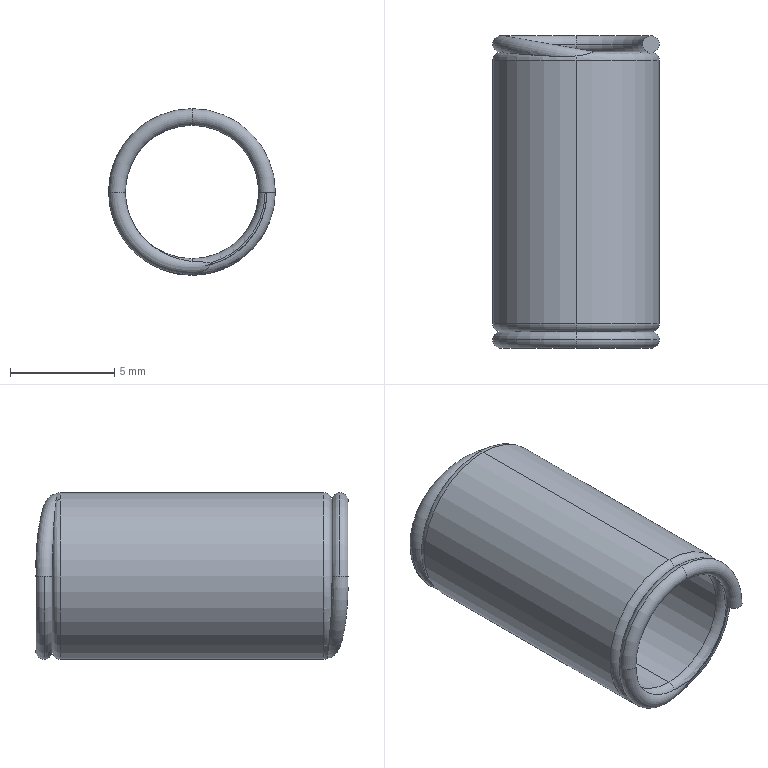Part | STEP file | 11-WT8_1511 | 1 solid | 30 faces | box 8 x 15 x 8 mm | volume 255.021 mm3 | torus 22 | cylinder 4 | plane 4 | commonest cylinder face diameters 6.4 x2 8 x2
STEP:
#1=CARTESIAN_POINT('',(0.,-7.1,4.));
#2=VERTEX_POINT('',#1);
#3=CARTESIAN_POINT('',(0.,-7.1,3.2));
#4=VERTEX_POINT('',#3);
#5=CARTESIAN_POINT('',(0.,-7.1,3.6));
#6=DIRECTION('',(1.,0.,0.));
#7=DIRECTION('',(0.,0.,-1.));
#8=AXIS2_PLACEMENT_3D('',#5,#6,#7);
#9=CIRCLE('',#8,0.4);
#10=EDGE_CURVE('',#2,#4,#9,.T.);
#11=ORIENTED_EDGE('',*,*,#10,.F.);
#12=CARTESIAN_POINT('',(-4.,-7.1,0.));
#13=VERTEX_POINT('',#12);
#14=CARTESIAN_POINT('',(0.,-7.1,0.));
#15=DIRECTION('',(0.,-1.,0.));
#16=DIRECTION('',(0.,0.,-1.));
#17=AXIS2_PLACEMENT_3D('',#14,#15,#16);
#18=CIRCLE('',#17,4.);
#19=EDGE_CURVE('',#2,#13,#18,.T.);
#20=ORIENTED_EDGE('',*,*,#19,.T.);
#21=CARTESIAN_POINT('',(-3.2,-7.1,0.));
#22=VERTEX_POINT('',#21);
#23=CARTESIAN_POINT('',(-3.6,-7.1,0.));
#24=DIRECTION('',(0.,0.,1.));
#25=DIRECTION('',(1.,0.,0.));
#26=AXIS2_PLACEMENT_3D('',#23,#24,#25);
#27=CIRCLE('',#26,0.4);
#28=EDGE_CURVE('',#13,#22,#27,.T.);
#29=ORIENTED_EDGE('',*,*,#28,.T.);
#30=CARTESIAN_POINT('',(0.,-7.1,0.));
#31=DIRECTION('',(0.,-1.,0.));
#32=DIRECTION('',(0.,0.,-1.));
#33=AXIS2_PLACEMENT_3D('',#30,#31,#32);
#34=CIRCLE('',#33,3.2);
#35=EDGE_CURVE('',#4,#22,#34,.T.);
#36=ORIENTED_EDGE('',*,*,#35,.F.);
#37=EDGE_LOOP('',(#11,#20,#29,#36));
#38=FACE_OUTER_BOUND('',#37,.T.);
#39=CARTESIAN_POINT('',(0.,-7.1,0.));
#40=DIRECTION('',(0.,-1.,0.));
#41=DIRECTION('',(0.,0.,-1.));
#42=AXIS2_PLACEMENT_3D('',#39,#40,#41);
#43=TOROIDAL_SURFACE('',#42,3.6,0.4);
#44=ADVANCED_FACE('',(#38),#43,.T.);
#45=CARTESIAN_POINT('',(0.,-6.7,3.6));
#46=VERTEX_POINT('',#45);
#47=CARTESIAN_POINT('',(0.,-7.1,3.6));
#48=DIRECTION('',(1.,0.,0.));
#49=DIRECTION('',(0.,0.,-1.));
#50=AXIS2_PLACEMENT_3D('',#47,#48,#49);
#51=CIRCLE('',#50,0.4);
#52=EDGE_CURVE('',#4,#46,#51,.T.);
#53=ORIENTED_EDGE('',*,*,#52,.F.);
#54=ORIENTED_EDGE('',*,*,#35,.T.);
#55=CARTESIAN_POINT('',(0.,-6.807,-3.328));
#56=VERTEX_POINT('',#55);
#57=CARTESIAN_POINT('',(0.,-6.807,-3.328));
#58=CARTESIAN_POINT('',(-0.4208,-6.848,-3.284));
#59=CARTESIAN_POINT('',(-0.8292,-6.886,-3.181));
#60=CARTESIAN_POINT('',(-1.409,-6.939,-2.918));
#61=CARTESIAN_POINT('',(-1.592,-6.956,-2.814));
#62=CARTESIAN_POINT('',(-1.937,-6.987,-2.576));
#63=CARTESIAN_POINT('',(-2.101,-7.002,-2.439));
#64=CARTESIAN_POINT('',(-2.398,-7.029,-2.139));
#65=CARTESIAN_POINT('',(-2.531,-7.041,-1.976));
#66=CARTESIAN_POINT('',(-2.766,-7.062,-1.627));
#67=CARTESIAN_POINT('',(-2.868,-7.071,-1.438));
#68=CARTESIAN_POINT('',(-3.031,-7.085,-1.047));
#69=CARTESIAN_POINT('',(-3.095,-7.091,-0.8424));
#70=CARTESIAN_POINT('',(-3.179,-7.098,-0.4249));
#71=CARTESIAN_POINT('',(-3.2,-7.1,-0.2096));
#72=CARTESIAN_POINT('',(-3.2,-7.1,0.));
#73=B_SPLINE_CURVE_WITH_KNOTS('',3,(#57,#58,#59,#60,#61,#62,#63,#64,#65,#66,#67,#68,#69,#70,#71,#72),.UNSPECIFIED.,.F.,.F.,(4,2,2,2,2,2,2,4),(0.001402,0.002659,0.003288,0.003917,0.004545,0.005174,0.005803,0.006431),.UNSPECIFIED.);
#74=EDGE_CURVE('',#56,#22,#73,.T.);
#75=ORIENTED_EDGE('',*,*,#74,.F.);
#76=CARTESIAN_POINT('',(0.,-6.7,-3.6));
#77=VERTEX_POINT('',#76);
#78=CARTESIAN_POINT('',(0.,-7.1,-3.6));
#79=DIRECTION('',(-1.,0.,0.));
#80=DIRECTION('',(0.,0.,1.));
#81=AXIS2_PLACEMENT_3D('',#78,#79,#80);
#82=CIRCLE('',#81,0.4);
#83=EDGE_CURVE('',#56,#77,#82,.T.);
#84=ORIENTED_EDGE('',*,*,#83,.T.);
#85=CARTESIAN_POINT('',(0.,-6.7,0.));
#86=DIRECTION('',(0.,1.,0.));
#87=DIRECTION('',(0.,0.,1.));
#88=AXIS2_PLACEMENT_3D('',#85,#86,#87);
#89=CIRCLE('',#88,3.6);
#90=EDGE_CURVE('',#77,#46,#89,.T.);
#91=ORIENTED_EDGE('',*,*,#90,.T.);
#92=EDGE_LOOP('',(#53,#54,#75,#84,#91));
#93=FACE_OUTER_BOUND('',#92,.T.);
#94=CARTESIAN_POINT('',(0.,-7.1,0.));
#95=DIRECTION('',(0.,-1.,0.));
#96=DIRECTION('',(0.,0.,-1.));
#97=AXIS2_PLACEMENT_3D('',#94,#95,#96);
#98=TOROIDAL_SURFACE('',#97,3.6,0.4);
#99=ADVANCED_FACE('',(#93),#98,.T.);
#100=CARTESIAN_POINT('',(0.,7.1,-4.));
#101=VERTEX_POINT('',#100);
#102=CARTESIAN_POINT('',(0.,7.1,-3.2));
#103=VERTEX_POINT('',#102);
#104=CARTESIAN_POINT('',(0.,7.1,-3.6));
#105=DIRECTION('',(1.,0.,0.));
#106=DIRECTION('',(0.,0.,-1.));
#107=AXIS2_PLACEMENT_3D('',#104,#105,#106);
#108=CIRCLE('',#107,0.4);
#109=EDGE_CURVE('',#101,#103,#108,.T.);
#110=ORIENTED_EDGE('',*,*,#109,.F.);
#111=CARTESIAN_POINT('',(-4.,7.1,0.));
#112=VERTEX_POINT('',#111);
#113=CARTESIAN_POINT('',(0.,7.1,0.));
#114=DIRECTION('',(0.,1.,0.));
#115=DIRECTION('',(0.,0.,1.));
#116=AXIS2_PLACEMENT_3D('',#113,#114,#115);
#117=CIRCLE('',#116,4.);
#118=EDGE_CURVE('',#101,#112,#117,.T.);
#119=ORIENTED_EDGE('',*,*,#118,.T.);
#120=CARTESIAN_POINT('',(-3.2,7.1,0.));
#121=VERTEX_POINT('',#120);
#122=CARTESIAN_POINT('',(-3.6,7.1,0.));
#123=DIRECTION('',(0.,0.,1.));
#124=DIRECTION('',(1.,0.,0.));
#125=AXIS2_PLACEMENT_3D('',#122,#123,#124);
#126=CIRCLE('',#125,0.4);
#127=EDGE_CURVE('',#121,#112,#126,.T.);
#128=ORIENTED_EDGE('',*,*,#127,.F.);
#129=CARTESIAN_POINT('',(0.,7.1,0.));
#130=DIRECTION('',(0.,1.,0.));
#131=DIRECTION('',(0.,0.,1.));
#132=AXIS2_PLACEMENT_3D('',#129,#130,#131);
#133=CIRCLE('',#132,3.2);
#134=EDGE_CURVE('',#103,#121,#133,.T.);
#135=ORIENTED_EDGE('',*,*,#134,.F.);
#136=EDGE_LOOP('',(#110,#119,#128,#135));
#137=FACE_OUTER_BOUND('',#136,.T.);
#138=CARTESIAN_POINT('',(0.,7.1,0.));
#139=DIRECTION('',(0.,1.,0.));
#140=DIRECTION('',(0.,0.,1.));
#141=AXIS2_PLACEMENT_3D('',#138,#139,#140);
#142=TOROIDAL_SURFACE('',#141,3.6,0.4);
#143=ADVANCED_FACE('',(#137),#142,.T.);
#144=CARTESIAN_POINT('',(0.,6.7,-3.6));
#145=VERTEX_POINT('',#144);
#146=CARTESIAN_POINT('',(0.,7.1,-3.6));
#147=DIRECTION('',(1.,0.,0.));
#148=DIRECTION('',(0.,0.,-1.));
#149=AXIS2_PLACEMENT_3D('',#146,#147,#148);
#150=CIRCLE('',#149,0.4);
#151=EDGE_CURVE('',#103,#145,#150,.T.);
#152=ORIENTED_EDGE('',*,*,#151,.F.);
#153=ORIENTED_EDGE('',*,*,#134,.T.);
#154=CARTESIAN_POINT('',(0.,6.807,3.328));
#155=VERTEX_POINT('',#154);
#156=CARTESIAN_POINT('',(-3.2,7.1,0.));
#157=CARTESIAN_POINT('',(-3.2,7.1,0.4264));
#158=CARTESIAN_POINT('',(-3.113,7.092,0.8528));
#159=CARTESIAN_POINT('',(-2.867,7.071,1.439));
#160=CARTESIAN_POINT('',(-2.765,7.062,1.628));
#161=CARTESIAN_POINT('',(-2.53,7.041,1.977));
#162=CARTESIAN_POINT('',(-2.397,7.029,2.139));
#163=CARTESIAN_POINT('',(-2.1,7.002,2.439));
#164=CARTESIAN_POINT('',(-1.936,6.987,2.576));
#165=CARTESIAN_POINT('',(-1.591,6.956,2.815));
#166=CARTESIAN_POINT('',(-1.408,6.939,2.918));
#167=CARTESIAN_POINT('',(-0.829,6.886,3.181));
#168=CARTESIAN_POINT('',(-0.4207,6.848,3.284));
#169=CARTESIAN_POINT('',(0.,6.807,3.328));
#170=B_SPLINE_CURVE_WITH_KNOTS('',3,(#156,#157,#158,#159,#160,#161,#162,#163,#164,#165,#166,#167,#168,#169),.UNSPECIFIED.,.F.,.F.,(4,2,2,2,2,2,4),(-0.00008421,0.001195,0.001834,0.002474,0.003113,0.003753,0.005032),.UNSPECIFIED.);
#171=EDGE_CURVE('',#121,#155,#170,.T.);
#172=ORIENTED_EDGE('',*,*,#171,.T.);
#173=CARTESIAN_POINT('',(0.,6.7,3.6));
#174=VERTEX_POINT('',#173);
#175=CARTESIAN_POINT('',(0.,7.1,3.6));
#176=DIRECTION('',(-1.,0.,0.));
#177=DIRECTION('',(0.,0.,1.));
#178=AXIS2_PLACEMENT_3D('',#175,#176,#177);
#179=CIRCLE('',#178,0.4);
#180=EDGE_CURVE('',#155,#174,#179,.T.);
#181=ORIENTED_EDGE('',*,*,#180,.T.);
#182=CARTESIAN_POINT('',(0.,6.7,0.));
#183=DIRECTION('',(0.,1.,0.));
#184=DIRECTION('',(0.,0.,1.));
#185=AXIS2_PLACEMENT_3D('',#182,#183,#184);
#186=CIRCLE('',#185,3.6);
#187=EDGE_CURVE('',#145,#174,#186,.T.);
#188=ORIENTED_EDGE('',*,*,#187,.F.);
#189=EDGE_LOOP('',(#152,#153,#172,#181,#188));
#190=FACE_OUTER_BOUND('',#189,.T.);
#191=CARTESIAN_POINT('',(0.,7.1,0.));
#192=DIRECTION('',(0.,1.,0.));
#193=DIRECTION('',(0.,0.,1.));
#194=AXIS2_PLACEMENT_3D('',#191,#192,#193);
#195=TOROIDAL_SURFACE('',#194,3.6,0.4);
#196=ADVANCED_FACE('',(#190),#195,.T.);
#197=CARTESIAN_POINT('',(3.2,7.1,0.));
#198=VERTEX_POINT('',#197);
#199=CARTESIAN_POINT('',(4.,7.1,0.));
#200=VERTEX_POINT('',#199);
#201=CARTESIAN_POINT('',(3.6,7.1,0.));
#202=DIRECTION('',(0.,0.,-1.));
#203=DIRECTION('',(-1.,0.,0.));
#204=AXIS2_PLACEMENT_3D('',#201,#202,#203);
#205=CIRCLE('',#204,0.4);
#206=EDGE_CURVE('',#198,#200,#205,.T.);
#207=ORIENTED_EDGE('',*,*,#206,.T.);
#208=CARTESIAN_POINT('',(0.,7.1,0.));
#209=DIRECTION('',(0.,1.,0.));
#210=DIRECTION('',(0.,0.,1.));
#211=AXIS2_PLACEMENT_3D('',#208,#209,#210);
#212=CIRCLE('',#211,4.);
#213=EDGE_CURVE('',#200,#101,#212,.T.);
#214=ORIENTED_EDGE('',*,*,#213,.T.);
#215=ORIENTED_EDGE('',*,*,#109,.T.);
#216=CARTESIAN_POINT('',(0.,7.1,0.));
#217=DIRECTION('',(0.,1.,0.));
#218=DIRECTION('',(0.,0.,1.));
#219=AXIS2_PLACEMENT_3D('',#216,#217,#218);
#220=CIRCLE('',#219,3.2);
#221=EDGE_CURVE('',#198,#103,#220,.T.);
#222=ORIENTED_EDGE('',*,*,#221,.F.);
#223=EDGE_LOOP('',(#207,#214,#215,#222));
#224=FACE_OUTER_BOUND('',#223,.T.);
#225=CARTESIAN_POINT('',(0.,7.1,0.));
#226=DIRECTION('',(0.,1.,0.));
#227=DIRECTION('',(0.,0.,1.));
#228=AXIS2_PLACEMENT_3D('',#225,#226,#227);
#229=TOROIDAL_SURFACE('',#228,3.6,0.4);
#230=ADVANCED_FACE('',(#224),#229,.T.);
#231=CARTESIAN_POINT('',(3.511,6.71,0.));
#232=VERTEX_POINT('',#231);
#233=CARTESIAN_POINT('',(3.6,7.1,0.));
#234=DIRECTION('',(0.,0.,-1.));
#235=DIRECTION('',(-1.,0.,0.));
#236=AXIS2_PLACEMENT_3D('',#233,#234,#235);
#237=CIRCLE('',#236,0.4);
#238=EDGE_CURVE('',#232,#198,#237,.T.);
#239=ORIENTED_EDGE('',*,*,#238,.T.);
#240=ORIENTED_EDGE('',*,*,#221,.T.);
#241=ORIENTED_EDGE('',*,*,#151,.T.);
#242=CARTESIAN_POINT('',(0.,6.7,0.));
#243=DIRECTION('',(0.,1.,0.));
#244=DIRECTION('',(0.,0.,1.));
#245=AXIS2_PLACEMENT_3D('',#242,#243,#244);
#246=CIRCLE('',#245,3.6);
#247=EDGE_CURVE('',#174,#145,#246,.T.);
#248=ORIENTED_EDGE('',*,*,#247,.F.);
#249=ORIENTED_EDGE('',*,*,#180,.F.);
#250=CARTESIAN_POINT('',(0.9125,6.71,3.39));
#251=VERTEX_POINT('',#250);
#252=CARTESIAN_POINT('',(0.,6.807,3.328));
#253=CARTESIAN_POINT('',(0.152,6.792,3.344));
#254=CARTESIAN_POINT('',(0.3044,6.777,3.352));
#255=CARTESIAN_POINT('',(0.5334,6.753,3.359));
#256=CARTESIAN_POINT('',(0.6097,6.745,3.36));
#257=CARTESIAN_POINT('',(0.724,6.733,3.364));
#258=CARTESIAN_POINT('',(0.7621,6.729,3.366));
#259=CARTESIAN_POINT('',(0.838,6.72,3.373));
#260=CARTESIAN_POINT('',(0.8766,6.715,3.377));
#261=CARTESIAN_POINT('',(0.9125,6.71,3.39));
#262=B_SPLINE_CURVE_WITH_KNOTS('',3,(#252,#253,#254,#255,#256,#257,#258,#259,#260,#261),.UNSPECIFIED.,.F.,.F.,(4,2,2,2,4),(0.005032,0.005494,0.005725,0.005841,0.005956),.UNSPECIFIED.);
#263=EDGE_CURVE('',#155,#251,#262,.T.);
#264=ORIENTED_EDGE('',*,*,#263,.T.);
#265=CARTESIAN_POINT('',(0.,6.71,0.));
#266=DIRECTION('',(0.,1.,0.));
#267=DIRECTION('',(0.,0.,1.));
#268=AXIS2_PLACEMENT_3D('',#265,#266,#267);
#269=CIRCLE('',#268,3.511);
#270=EDGE_CURVE('',#251,#232,#269,.T.);
#271=ORIENTED_EDGE('',*,*,#270,.T.);
#272=EDGE_LOOP('',(#239,#240,#241,#248,#249,#264,#271));
#273=FACE_OUTER_BOUND('',#272,.T.);
#274=CARTESIAN_POINT('',(0.,7.1,0.));
#275=DIRECTION('',(0.,1.,0.));
#276=DIRECTION('',(0.,0.,1.));
#277=AXIS2_PLACEMENT_3D('',#274,#275,#276);
#278=TOROIDAL_SURFACE('',#277,3.6,0.4);
#279=ADVANCED_FACE('',(#273),#278,.T.);
#280=CARTESIAN_POINT('',(4.,-7.1,0.));
#281=VERTEX_POINT('',#280);
#282=CARTESIAN_POINT('',(3.2,-7.1,0.));
#283=VERTEX_POINT('',#282);
#284=CARTESIAN_POINT('',(3.6,-7.1,0.));
#285=DIRECTION('',(0.,0.,-1.));
#286=DIRECTION('',(-1.,0.,0.));
#287=AXIS2_PLACEMENT_3D('',#284,#285,#286);
#288=CIRCLE('',#287,0.4);
#289=EDGE_CURVE('',#281,#283,#288,.T.);
#290=ORIENTED_EDGE('',*,*,#289,.F.);
#291=CARTESIAN_POINT('',(0.,-7.1,0.));
#292=DIRECTION('',(0.,-1.,0.));
#293=DIRECTION('',(0.,0.,-1.));
#294=AXIS2_PLACEMENT_3D('',#291,#292,#293);
#295=CIRCLE('',#294,4.);
#296=EDGE_CURVE('',#281,#2,#295,.T.);
#297=ORIENTED_EDGE('',*,*,#296,.T.);
#298=ORIENTED_EDGE('',*,*,#10,.T.);
#299=CARTESIAN_POINT('',(0.,-7.1,0.));
#300=DIRECTION('',(0.,-1.,0.));
#301=DIRECTION('',(0.,0.,-1.));
#302=AXIS2_PLACEMENT_3D('',#299,#300,#301);
#303=CIRCLE('',#302,3.2);
#304=EDGE_CURVE('',#283,#4,#303,.T.);
#305=ORIENTED_EDGE('',*,*,#304,.F.);
#306=EDGE_LOOP('',(#290,#297,#298,#305));
#307=FACE_OUTER_BOUND('',#306,.T.);
#308=CARTESIAN_POINT('',(0.,-7.1,0.));
#309=DIRECTION('',(0.,-1.,0.));
#310=DIRECTION('',(0.,0.,-1.));
#311=AXIS2_PLACEMENT_3D('',#308,#309,#310);
#312=TOROIDAL_SURFACE('',#311,3.6,0.4);
#313=ADVANCED_FACE('',(#307),#312,.T.);
#314=CARTESIAN_POINT('',(3.511,-6.71,0.));
#315=VERTEX_POINT('',#314);
#316=CARTESIAN_POINT('',(3.6,-7.1,0.));
#317=DIRECTION('',(0.,0.,-1.));
#318=DIRECTION('',(-1.,0.,0.));
#319=AXIS2_PLACEMENT_3D('',#316,#317,#318);
#320=CIRCLE('',#319,0.4);
#321=EDGE_CURVE('',#283,#315,#320,.T.);
#322=ORIENTED_EDGE('',*,*,#321,.F.);
#323=ORIENTED_EDGE('',*,*,#304,.T.);
#324=ORIENTED_EDGE('',*,*,#52,.T.);
#325=CARTESIAN_POINT('',(0.,-6.7,0.));
#326=DIRECTION('',(0.,1.,0.));
#327=DIRECTION('',(0.,0.,1.));
#328=AXIS2_PLACEMENT_3D('',#325,#326,#327);
#329=CIRCLE('',#328,3.6);
#330=EDGE_CURVE('',#46,#77,#329,.T.);
#331=ORIENTED_EDGE('',*,*,#330,.T.);
#332=ORIENTED_EDGE('',*,*,#83,.F.);
#333=CARTESIAN_POINT('',(0.9125,-6.71,-3.39));
#334=VERTEX_POINT('',#333);
#335=CARTESIAN_POINT('',(0.9125,-6.71,-3.39));
#336=CARTESIAN_POINT('',(0.8766,-6.715,-3.377));
#337=CARTESIAN_POINT('',(0.838,-6.72,-3.373));
#338=CARTESIAN_POINT('',(0.7621,-6.729,-3.366));
#339=CARTESIAN_POINT('',(0.724,-6.733,-3.364));
#340=CARTESIAN_POINT('',(0.6097,-6.745,-3.36));
#341=CARTESIAN_POINT('',(0.5334,-6.753,-3.359));
#342=CARTESIAN_POINT('',(0.3044,-6.777,-3.352));
#343=CARTESIAN_POINT('',(0.152,-6.792,-3.344));
#344=CARTESIAN_POINT('',(0.,-6.807,-3.328));
#345=B_SPLINE_CURVE_WITH_KNOTS('',3,(#335,#336,#337,#338,#339,#340,#341,#342,#343,#344),.UNSPECIFIED.,.F.,.F.,(4,2,2,2,4),(0.0004938,0.0006073,0.0007209,0.0009479,0.001402),.UNSPECIFIED.);
#346=EDGE_CURVE('',#334,#56,#345,.T.);
#347=ORIENTED_EDGE('',*,*,#346,.F.);
#348=CARTESIAN_POINT('',(0.,-6.71,0.));
#349=DIRECTION('',(0.,-1.,0.));
#350=DIRECTION('',(0.,0.,-1.));
#351=AXIS2_PLACEMENT_3D('',#348,#349,#350);
#352=CIRCLE('',#351,3.511);
#353=EDGE_CURVE('',#334,#315,#352,.T.);
#354=ORIENTED_EDGE('',*,*,#353,.T.);
#355=EDGE_LOOP('',(#322,#323,#324,#331,#332,#347,#354));
#356=FACE_OUTER_BOUND('',#355,.T.);
#357=CARTESIAN_POINT('',(0.,-7.1,0.));
#358=DIRECTION('',(0.,-1.,0.));
#359=DIRECTION('',(0.,0.,-1.));
#360=AXIS2_PLACEMENT_3D('',#357,#358,#359);
#361=TOROIDAL_SURFACE('',#360,3.6,0.4);
#362=ADVANCED_FACE('',(#356),#361,.T.);
#363=ORIENTED_EDGE('',*,*,#247,.T.);
#364=CARTESIAN_POINT('',(0.,6.3,-3.2));
#365=VERTEX_POINT('',#364);
#366=CARTESIAN_POINT('',(0.,6.3,-3.6));
#367=DIRECTION('',(1.,0.,0.));
#368=DIRECTION('',(0.,0.,-1.));
#369=AXIS2_PLACEMENT_3D('',#366,#367,#368);
#370=CIRCLE('',#369,0.4);
#371=EDGE_CURVE('',#145,#365,#370,.T.);
#372=ORIENTED_EDGE('',*,*,#371,.T.);
#373=CARTESIAN_POINT('',(0.,6.3,3.2));
#374=VERTEX_POINT('',#373);
#375=CARTESIAN_POINT('',(0.,6.3,0.));
#376=DIRECTION('',(0.,1.,0.));
#377=DIRECTION('',(0.,0.,1.));
#378=AXIS2_PLACEMENT_3D('',#375,#376,#377);
#379=CIRCLE('',#378,3.2);
#380=EDGE_CURVE('',#374,#365,#379,.T.);
#381=ORIENTED_EDGE('',*,*,#380,.F.);
#382=CARTESIAN_POINT('',(0.,6.3,3.6));
#383=DIRECTION('',(-1.,0.,0.));
#384=DIRECTION('',(0.,0.,1.));
#385=AXIS2_PLACEMENT_3D('',#382,#383,#384);
#386=CIRCLE('',#385,0.4);
#387=EDGE_CURVE('',#174,#374,#386,.T.);
#388=ORIENTED_EDGE('',*,*,#387,.F.);
#389=EDGE_LOOP('',(#363,#372,#381,#388));
#390=FACE_OUTER_BOUND('',#389,.T.);
#391=CARTESIAN_POINT('',(0.,6.3,0.));
#392=DIRECTION('',(0.,1.,0.));
#393=DIRECTION('',(0.,0.,1.));
#394=AXIS2_PLACEMENT_3D('',#391,#392,#393);
#395=TOROIDAL_SURFACE('',#394,3.6,0.4);
#396=ADVANCED_FACE('',(#390),#395,.T.);
#397=CARTESIAN_POINT('',(0.,-6.3,-3.2));
#398=VERTEX_POINT('',#397);
#399=CARTESIAN_POINT('',(0.,-6.3,3.2));
#400=VERTEX_POINT('',#399);
#401=CARTESIAN_POINT('',(0.,-6.3,0.));
#402=DIRECTION('',(0.,1.,0.));
#403=DIRECTION('',(0.,0.,1.));
#404=AXIS2_PLACEMENT_3D('',#401,#402,#403);
#405=CIRCLE('',#404,3.2);
#406=EDGE_CURVE('',#398,#400,#405,.T.);
#407=ORIENTED_EDGE('',*,*,#406,.F.);
#408=CARTESIAN_POINT('',(0.,-7.5,-3.2));
#409=DIRECTION('',(0.,1.,0.));
#410=VECTOR('',#409,1000.);
#411=LINE('',#408,#410);
#412=EDGE_CURVE('',#398,#365,#411,.T.);
#413=ORIENTED_EDGE('',*,*,#412,.T.);
#414=CARTESIAN_POINT('',(0.,6.3,0.));
#415=DIRECTION('',(0.,1.,0.));
#416=DIRECTION('',(0.,0.,1.));
#417=AXIS2_PLACEMENT_3D('',#414,#415,#416);
#418=CIRCLE('',#417,3.2);
#419=EDGE_CURVE('',#365,#374,#418,.T.);
#420=ORIENTED_EDGE('',*,*,#419,.T.);
#421=CARTESIAN_POINT('',(0.,-7.5,3.2));
#422=DIRECTION('',(0.,1.,0.));
#423=VECTOR('',#422,1000.);
#424=LINE('',#421,#423);
#425=EDGE_CURVE('',#400,#374,#424,.T.);
#426=ORIENTED_EDGE('',*,*,#425,.F.);
#427=EDGE_LOOP('',(#407,#413,#420,#426));
#428=FACE_OUTER_BOUND('',#427,.T.);
#429=CARTESIAN_POINT('',(0.,-7.5,0.));
#430=DIRECTION('',(0.,1.,0.));
#431=DIRECTION('',(0.,0.,1.));
#432=AXIS2_PLACEMENT_3D('',#429,#430,#431);
#433=CYLINDRICAL_SURFACE('',#432,3.2);
#434=ADVANCED_FACE('',(#428),#433,.F.);
#435=CARTESIAN_POINT('',(0.,-6.3,0.));
#436=DIRECTION('',(0.,1.,0.));
#437=DIRECTION('',(0.,0.,1.));
#438=AXIS2_PLACEMENT_3D('',#435,#436,#437);
#439=CIRCLE('',#438,3.2);
#440=EDGE_CURVE('',#400,#398,#439,.T.);
#441=ORIENTED_EDGE('',*,*,#440,.T.);
#442=CARTESIAN_POINT('',(0.,-6.3,-3.6));
#443=DIRECTION('',(1.,0.,0.));
#444=DIRECTION('',(0.,0.,-1.));
#445=AXIS2_PLACEMENT_3D('',#442,#443,#444);
#446=CIRCLE('',#445,0.4);
#447=EDGE_CURVE('',#398,#77,#446,.T.);
#448=ORIENTED_EDGE('',*,*,#447,.T.);
#449=ORIENTED_EDGE('',*,*,#330,.F.);
#450=CARTESIAN_POINT('',(0.,-6.3,3.6));
#451=DIRECTION('',(-1.,0.,0.));
#452=DIRECTION('',(0.,0.,1.));
#453=AXIS2_PLACEMENT_3D('',#450,#451,#452);
#454=CIRCLE('',#453,0.4);
#455=EDGE_CURVE('',#400,#46,#454,.T.);
#456=ORIENTED_EDGE('',*,*,#455,.F.);
#457=EDGE_LOOP('',(#441,#448,#449,#456));
#458=FACE_OUTER_BOUND('',#457,.T.);
#459=CARTESIAN_POINT('',(0.,-6.3,0.));
#460=DIRECTION('',(0.,1.,0.));
#461=DIRECTION('',(0.,0.,1.));
#462=AXIS2_PLACEMENT_3D('',#459,#460,#461);
#463=TOROIDAL_SURFACE('',#462,3.6,0.4);
#464=ADVANCED_FACE('',(#458),#463,.T.);
#465=ORIENTED_EDGE('',*,*,#296,.F.);
#466=CARTESIAN_POINT('',(3.663,-6.705,0.));
#467=VERTEX_POINT('',#466);
#468=CARTESIAN_POINT('',(3.6,-7.1,0.));
#469=DIRECTION('',(0.,0.,-1.));
#470=DIRECTION('',(-1.,0.,0.));
#471=AXIS2_PLACEMENT_3D('',#468,#469,#470);
#472=CIRCLE('',#471,0.4);
#473=EDGE_CURVE('',#467,#281,#472,.T.);
#474=ORIENTED_EDGE('',*,*,#473,.F.);
#475=CARTESIAN_POINT('',(0.,-6.705,3.663));
#476=VERTEX_POINT('',#475);
#477=CARTESIAN_POINT('',(0.,-6.705,0.));
#478=DIRECTION('',(0.,-1.,0.));
#479=DIRECTION('',(0.,0.,-1.));
#480=AXIS2_PLACEMENT_3D('',#477,#478,#479);
#481=CIRCLE('',#480,3.663);
#482=EDGE_CURVE('',#467,#476,#481,.T.);
#483=ORIENTED_EDGE('',*,*,#482,.T.);
#484=CARTESIAN_POINT('',(0.,-7.1,3.6));
#485=DIRECTION('',(1.,0.,0.));
#486=DIRECTION('',(0.,0.,-1.));
#487=AXIS2_PLACEMENT_3D('',#484,#485,#486);
#488=CIRCLE('',#487,0.4);
#489=EDGE_CURVE('',#476,#2,#488,.T.);
#490=ORIENTED_EDGE('',*,*,#489,.T.);
#491=EDGE_LOOP('',(#465,#474,#483,#490));
#492=FACE_OUTER_BOUND('',#491,.T.);
#493=CARTESIAN_POINT('',(0.,-7.1,0.));
#494=DIRECTION('',(0.,-1.,0.));
#495=DIRECTION('',(0.,0.,-1.));
#496=AXIS2_PLACEMENT_3D('',#493,#494,#495);
#497=TOROIDAL_SURFACE('',#496,3.6,0.4);
#498=ADVANCED_FACE('',(#492),#497,.T.);
#499=ORIENTED_EDGE('',*,*,#213,.F.);
#500=CARTESIAN_POINT('',(3.663,6.705,0.));
#501=VERTEX_POINT('',#500);
#502=CARTESIAN_POINT('',(3.6,7.1,0.));
#503=DIRECTION('',(0.,0.,-1.));
#504=DIRECTION('',(-1.,0.,0.));
#505=AXIS2_PLACEMENT_3D('',#502,#503,#504);
#506=CIRCLE('',#505,0.4);
#507=EDGE_CURVE('',#200,#501,#506,.T.);
#508=ORIENTED_EDGE('',*,*,#507,.T.);
#509=CARTESIAN_POINT('',(0.,6.705,-3.663));
#510=VERTEX_POINT('',#509);
#511=CARTESIAN_POINT('',(0.,6.705,0.));
#512=DIRECTION('',(0.,-1.,0.));
#513=DIRECTION('',(0.,0.,1.));
#514=AXIS2_PLACEMENT_3D('',#511,#512,#513);
#515=CIRCLE('',#514,3.663);
#516=EDGE_CURVE('',#510,#501,#515,.T.);
#517=ORIENTED_EDGE('',*,*,#516,.F.);
#518=CARTESIAN_POINT('',(0.,7.1,-3.6));
#519=DIRECTION('',(1.,0.,0.));
#520=DIRECTION('',(0.,0.,-1.));
#521=AXIS2_PLACEMENT_3D('',#518,#519,#520);
#522=CIRCLE('',#521,0.4);
#523=EDGE_CURVE('',#510,#101,#522,.T.);
#524=ORIENTED_EDGE('',*,*,#523,.T.);
#525=EDGE_LOOP('',(#499,#508,#517,#524));
#526=FACE_OUTER_BOUND('',#525,.T.);
#527=CARTESIAN_POINT('',(0.,7.1,0.));
#528=DIRECTION('',(0.,1.,0.));
#529=DIRECTION('',(0.,0.,1.));
#530=AXIS2_PLACEMENT_3D('',#527,#528,#529);
#531=TOROIDAL_SURFACE('',#530,3.6,0.4);
#532=ADVANCED_FACE('',(#526),#531,.T.);
#533=CARTESIAN_POINT('',(0.8814,-6.71,-3.49));
#534=VERTEX_POINT('',#533);
#535=CARTESIAN_POINT('',(0.,-6.52,-3.94));
#536=VERTEX_POINT('',#535);
#537=CARTESIAN_POINT('',(0.8814,-6.71,-3.49));
#538=CARTESIAN_POINT('',(0.8282,-6.71,-3.56));
#539=CARTESIAN_POINT('',(0.7727,-6.698,-3.627));
#540=CARTESIAN_POINT('',(0.6454,-6.661,-3.743));
#541=CARTESIAN_POINT('',(0.5762,-6.637,-3.79));
#542=CARTESIAN_POINT('',(0.4239,-6.593,-3.863));
#543=CARTESIAN_POINT('',(0.3411,-6.572,-3.889));
#544=CARTESIAN_POINT('',(0.1735,-6.541,-3.924));
#545=CARTESIAN_POINT('',(0.08723,-6.529,-3.935));
#546=CARTESIAN_POINT('',(0.,-6.52,-3.94));
#547=B_SPLINE_CURVE_WITH_KNOTS('',3,(#537,#538,#539,#540,#541,#542,#543,#544,#545,#546),.UNSPECIFIED.,.F.,.F.,(4,2,2,2,4),(0.002419,0.002678,0.002938,0.003197,0.003457),.UNSPECIFIED.);
#548=EDGE_CURVE('',#534,#536,#547,.T.);
#549=ORIENTED_EDGE('',*,*,#548,.T.);
#550=CARTESIAN_POINT('',(0.,-6.31,-4.));
#551=VERTEX_POINT('',#550);
#552=CARTESIAN_POINT('',(0.,-6.31,-3.6));
#553=DIRECTION('',(1.,0.,0.));
#554=DIRECTION('',(0.,0.,-1.));
#555=AXIS2_PLACEMENT_3D('',#552,#553,#554);
#556=CIRCLE('',#555,0.4);
#557=EDGE_CURVE('',#536,#551,#556,.T.);
#558=ORIENTED_EDGE('',*,*,#557,.T.);
#559=CARTESIAN_POINT('',(0.,-6.31,4.));
#560=VERTEX_POINT('',#559);
#561=CARTESIAN_POINT('',(0.,-6.31,0.));
#562=DIRECTION('',(0.,1.,0.));
#563=DIRECTION('',(0.,0.,1.));
#564=AXIS2_PLACEMENT_3D('',#561,#562,#563);
#565=CIRCLE('',#564,4.);
#566=EDGE_CURVE('',#560,#551,#565,.T.);
#567=ORIENTED_EDGE('',*,*,#566,.F.);
#568=CARTESIAN_POINT('',(0.,-6.31,3.6));
#569=DIRECTION('',(-1.,0.,0.));
#570=DIRECTION('',(0.,0.,1.));
#571=AXIS2_PLACEMENT_3D('',#568,#569,#570);
#572=CIRCLE('',#571,0.4);
#573=EDGE_CURVE('',#476,#560,#572,.T.);
#574=ORIENTED_EDGE('',*,*,#573,.F.);
#575=ORIENTED_EDGE('',*,*,#482,.F.);
#576=CARTESIAN_POINT('',(3.6,-6.71,0.));
#577=VERTEX_POINT('',#576);
#578=CARTESIAN_POINT('',(3.6,-6.31,0.));
#579=DIRECTION('',(0.,0.,-1.));
#580=DIRECTION('',(-1.,0.,0.));
#581=AXIS2_PLACEMENT_3D('',#578,#579,#580);
#582=CIRCLE('',#581,0.4);
#583=EDGE_CURVE('',#467,#577,#582,.T.);
#584=ORIENTED_EDGE('',*,*,#583,.T.);
#585=CARTESIAN_POINT('',(0.,-6.71,0.));
#586=DIRECTION('',(0.,1.,0.));
#587=DIRECTION('',(0.,0.,1.));
#588=AXIS2_PLACEMENT_3D('',#585,#586,#587);
#589=CIRCLE('',#588,3.6);
#590=EDGE_CURVE('',#577,#534,#589,.T.);
#591=ORIENTED_EDGE('',*,*,#590,.T.);
#592=EDGE_LOOP('',(#549,#558,#567,#574,#575,#584,#591));
#593=FACE_OUTER_BOUND('',#592,.T.);
#594=CARTESIAN_POINT('',(0.,-6.31,0.));
#595=DIRECTION('',(0.,1.,0.));
#596=DIRECTION('',(0.,0.,1.));
#597=AXIS2_PLACEMENT_3D('',#594,#595,#596);
#598=TOROIDAL_SURFACE('',#597,3.6,0.4);
#599=ADVANCED_FACE('',(#593),#598,.T.);
#600=ORIENTED_EDGE('',*,*,#566,.T.);
#601=CARTESIAN_POINT('',(0.,6.31,-4.));
#602=VERTEX_POINT('',#601);
#603=CARTESIAN_POINT('',(0.,-6.71,-4.));
#604=DIRECTION('',(0.,1.,0.));
#605=VECTOR('',#604,1000.);
#606=LINE('',#603,#605);
#607=EDGE_CURVE('',#551,#602,#606,.T.);
#608=ORIENTED_EDGE('',*,*,#607,.T.);
#609=CARTESIAN_POINT('',(0.,6.31,4.));
#610=VERTEX_POINT('',#609);
#611=CARTESIAN_POINT('',(0.,6.31,0.));
#612=DIRECTION('',(0.,1.,0.));
#613=DIRECTION('',(0.,0.,1.));
#614=AXIS2_PLACEMENT_3D('',#611,#612,#613);
#615=CIRCLE('',#614,4.);
#616=EDGE_CURVE('',#610,#602,#615,.T.);
#617=ORIENTED_EDGE('',*,*,#616,.F.);
#618=CARTESIAN_POINT('',(0.,-6.71,4.));
#619=DIRECTION('',(0.,1.,0.));
#620=VECTOR('',#619,1000.);
#621=LINE('',#618,#620);
#622=EDGE_CURVE('',#560,#610,#621,.T.);
#623=ORIENTED_EDGE('',*,*,#622,.F.);
#624=EDGE_LOOP('',(#600,#608,#617,#623));
#625=FACE_OUTER_BOUND('',#624,.T.);
#626=CARTESIAN_POINT('',(0.,-6.71,0.));
#627=DIRECTION('',(0.,1.,0.));
#628=DIRECTION('',(0.,0.,1.));
#629=AXIS2_PLACEMENT_3D('',#626,#627,#628);
#630=CYLINDRICAL_SURFACE('',#629,4.);
#631=ADVANCED_FACE('',(#625),#630,.T.);
#632=ORIENTED_EDGE('',*,*,#616,.T.);
#633=CARTESIAN_POINT('',(0.,6.31,-3.6));
#634=DIRECTION('',(1.,0.,0.));
#635=DIRECTION('',(0.,0.,-1.));
#636=AXIS2_PLACEMENT_3D('',#633,#634,#635);
#637=CIRCLE('',#636,0.4);
#638=EDGE_CURVE('',#602,#510,#637,.T.);
#639=ORIENTED_EDGE('',*,*,#638,.T.);
#640=ORIENTED_EDGE('',*,*,#516,.T.);
#641=CARTESIAN_POINT('',(3.6,6.71,0.));
#642=VERTEX_POINT('',#641);
#643=CARTESIAN_POINT('',(3.6,6.31,0.));
#644=DIRECTION('',(0.,0.,-1.));
#645=DIRECTION('',(-1.,0.,0.));
#646=AXIS2_PLACEMENT_3D('',#643,#644,#645);
#647=CIRCLE('',#646,0.4);
#648=EDGE_CURVE('',#642,#501,#647,.T.);
#649=ORIENTED_EDGE('',*,*,#648,.F.);
#650=CARTESIAN_POINT('',(0.8814,6.71,3.49));
#651=VERTEX_POINT('',#650);
#652=CARTESIAN_POINT('',(0.,6.71,0.));
#653=DIRECTION('',(0.,1.,0.));
#654=DIRECTION('',(0.,0.,1.));
#655=AXIS2_PLACEMENT_3D('',#652,#653,#654);
#656=CIRCLE('',#655,3.6);
#657=EDGE_CURVE('',#651,#642,#656,.T.);
#658=ORIENTED_EDGE('',*,*,#657,.F.);
#659=CARTESIAN_POINT('',(0.,6.52,3.94));
#660=VERTEX_POINT('',#659);
#661=CARTESIAN_POINT('',(0.,6.52,3.94));
#662=CARTESIAN_POINT('',(0.1732,6.538,3.93));
#663=CARTESIAN_POINT('',(0.3465,6.57,3.899));
#664=CARTESIAN_POINT('',(0.5755,6.637,3.79));
#665=CARTESIAN_POINT('',(0.6463,6.661,3.742));
#666=CARTESIAN_POINT('',(0.7716,6.698,3.628));
#667=CARTESIAN_POINT('',(0.8281,6.71,3.56));
#668=CARTESIAN_POINT('',(0.8814,6.71,3.49));
#669=B_SPLINE_CURVE_WITH_KNOTS('',3,(#661,#662,#663,#664,#665,#666,#667,#668),.UNSPECIFIED.,.F.,.F.,(4,2,2,4),(0.006073,0.006595,0.006856,0.007117),.UNSPECIFIED.);
#670=EDGE_CURVE('',#660,#651,#669,.T.);
#671=ORIENTED_EDGE('',*,*,#670,.F.);
#672=CARTESIAN_POINT('',(0.,6.31,3.6));
#673=DIRECTION('',(-1.,0.,0.));
#674=DIRECTION('',(0.,0.,1.));
#675=AXIS2_PLACEMENT_3D('',#672,#673,#674);
#676=CIRCLE('',#675,0.4);
#677=EDGE_CURVE('',#610,#660,#676,.T.);
#678=ORIENTED_EDGE('',*,*,#677,.F.);
#679=EDGE_LOOP('',(#632,#639,#640,#649,#658,#671,#678));
#680=FACE_OUTER_BOUND('',#679,.T.);
#681=CARTESIAN_POINT('',(0.,6.31,0.));
#682=DIRECTION('',(0.,1.,0.));
#683=DIRECTION('',(0.,0.,1.));
#684=AXIS2_PLACEMENT_3D('',#681,#682,#683);
#685=TOROIDAL_SURFACE('',#684,3.6,0.4);
#686=ADVANCED_FACE('',(#680),#685,.T.);
#687=ORIENTED_EDGE('',*,*,#270,.F.);
#688=CARTESIAN_POINT('',(0.8814,6.71,3.49));
#689=CARTESIAN_POINT('',(0.8924,6.71,3.476));
#690=CARTESIAN_POINT('',(0.9022,6.71,3.461));
#691=CARTESIAN_POINT('',(0.9151,6.71,3.427));
#692=CARTESIAN_POINT('',(0.9176,6.71,3.408));
#693=CARTESIAN_POINT('',(0.9125,6.71,3.39));
#694=B_SPLINE_CURVE_WITH_KNOTS('',3,(#688,#689,#690,#691,#692,#693),.UNSPECIFIED.,.F.,.F.,(4,2,4),(0.02562,0.02567,0.02572),.UNSPECIFIED.);
#695=EDGE_CURVE('',#651,#251,#694,.T.);
#696=ORIENTED_EDGE('',*,*,#695,.F.);
#697=ORIENTED_EDGE('',*,*,#657,.T.);
#698=CARTESIAN_POINT('',(0.,6.71,0.));
#699=DIRECTION('',(1.,0.,0.));
#700=VECTOR('',#699,1000.);
#701=LINE('',#698,#700);
#702=EDGE_CURVE('',#232,#642,#701,.T.);
#703=ORIENTED_EDGE('',*,*,#702,.F.);
#704=EDGE_LOOP('',(#687,#696,#697,#703));
#705=FACE_OUTER_BOUND('',#704,.T.);
#706=CARTESIAN_POINT('',(0.,6.71,0.));
#707=DIRECTION('',(0.,-1.,0.));
#708=DIRECTION('',(0.,0.,-1.));
#709=AXIS2_PLACEMENT_3D('',#706,#707,#708);
#710=PLANE('',#709);
#711=ADVANCED_FACE('',(#705),#710,.F.);
#712=ORIENTED_EDGE('',*,*,#353,.F.);
#713=CARTESIAN_POINT('',(0.9125,-6.71,-3.39));
#714=CARTESIAN_POINT('',(0.9177,-6.71,-3.408));
#715=CARTESIAN_POINT('',(0.9151,-6.71,-3.427));
#716=CARTESIAN_POINT('',(0.9022,-6.71,-3.461));
#717=CARTESIAN_POINT('',(0.8924,-6.71,-3.476));
#718=CARTESIAN_POINT('',(0.8814,-6.71,-3.49));
#719=B_SPLINE_CURVE_WITH_KNOTS('',3,(#713,#714,#715,#716,#717,#718),.UNSPECIFIED.,.F.,.F.,(4,2,4),(0.0009489,0.001002,0.001056),.UNSPECIFIED.);
#720=EDGE_CURVE('',#334,#534,#719,.T.);
#721=ORIENTED_EDGE('',*,*,#720,.T.);
#722=ORIENTED_EDGE('',*,*,#590,.F.);
#723=CARTESIAN_POINT('',(3.6,-6.71,0.));
#724=DIRECTION('',(-1.,0.,0.));
#725=VECTOR('',#724,1000.);
#726=LINE('',#723,#725);
#727=EDGE_CURVE('',#577,#315,#726,.T.);
#728=ORIENTED_EDGE('',*,*,#727,.T.);
#729=EDGE_LOOP('',(#712,#721,#722,#728));
#730=FACE_OUTER_BOUND('',#729,.T.);
#731=CARTESIAN_POINT('',(3.6,-6.71,0.));
#732=DIRECTION('',(0.,1.,0.));
#733=DIRECTION('',(0.,0.,1.));
#734=AXIS2_PLACEMENT_3D('',#731,#732,#733);
#735=PLANE('',#734);
#736=ADVANCED_FACE('',(#730),#735,.F.);
#737=ORIENTED_EDGE('',*,*,#171,.F.);
#738=ORIENTED_EDGE('',*,*,#127,.T.);
#739=CARTESIAN_POINT('',(-3.663,6.705,0.));
#740=VERTEX_POINT('',#739);
#741=CARTESIAN_POINT('',(-3.6,7.1,0.));
#742=DIRECTION('',(0.,0.,1.));
#743=DIRECTION('',(1.,0.,0.));
#744=AXIS2_PLACEMENT_3D('',#741,#742,#743);
#745=CIRCLE('',#744,0.4);
#746=EDGE_CURVE('',#112,#740,#745,.T.);
#747=ORIENTED_EDGE('',*,*,#746,.T.);
#748=CARTESIAN_POINT('',(-3.663,6.705,0.));
#749=CARTESIAN_POINT('',(-3.663,6.705,0.2536));
#750=CARTESIAN_POINT('',(-3.652,6.703,0.5064));
#751=CARTESIAN_POINT('',(-3.584,6.694,1.009));
#752=CARTESIAN_POINT('',(-3.527,6.687,1.254));
#753=CARTESIAN_POINT('',(-3.366,6.67,1.728));
#754=CARTESIAN_POINT('',(-3.26,6.66,1.959));
#755=CARTESIAN_POINT('',(-3.004,6.636,2.394));
#756=CARTESIAN_POINT('',(-2.855,6.623,2.594));
#757=CARTESIAN_POINT('',(-2.517,6.595,2.965));
#758=CARTESIAN_POINT('',(-2.326,6.58,3.135));
#759=CARTESIAN_POINT('',(-1.919,6.551,3.427));
#760=CARTESIAN_POINT('',(-1.701,6.537,3.551));
#761=CARTESIAN_POINT('',(-1.238,6.512,3.755));
#762=CARTESIAN_POINT('',(-0.9974,6.501,3.831));
#763=CARTESIAN_POINT('',(-0.6298,6.496,3.906));
#764=CARTESIAN_POINT('',(-0.5057,6.495,3.924));
#765=CARTESIAN_POINT('',(-0.2542,6.501,3.945));
#766=CARTESIAN_POINT('',(-0.1259,6.508,3.948));
#767=CARTESIAN_POINT('',(0.,6.52,3.94));
#768=B_SPLINE_CURVE_WITH_KNOTS('',3,(#748,#749,#750,#751,#752,#753,#754,#755,#756,#757,#758,#759,#760,#761,#762,#763,#764,#765,#766,#767),.UNSPECIFIED.,.F.,.F.,(4,2,2,2,2,2,2,2,2,4),(0.0000002,0.0007593,0.001518,0.002278,0.003037,0.003796,0.004555,0.005314,0.005693,0.006073),.UNSPECIFIED.);
#769=EDGE_CURVE('',#740,#660,#768,.T.);
#770=ORIENTED_EDGE('',*,*,#769,.T.);
#771=ORIENTED_EDGE('',*,*,#670,.T.);
#772=ORIENTED_EDGE('',*,*,#695,.T.);
#773=ORIENTED_EDGE('',*,*,#263,.F.);
#774=EDGE_LOOP('',(#737,#738,#747,#770,#771,#772,#773));
#775=FACE_OUTER_BOUND('',#774,.T.);
#776=CARTESIAN_POINT('',(-0.1086,6.484,0.));
#777=DIRECTION('',(-0.1736,-0.9848,0.));
#778=DIRECTION('',(0.9848,-0.1736,0.));
#779=AXIS2_PLACEMENT_3D('',#776,#777,#778);
#780=TOROIDAL_SURFACE('',#779,3.545,0.4);
#781=ADVANCED_FACE('',(#775),#780,.T.);
#782=ORIENTED_EDGE('',*,*,#720,.F.);
#783=ORIENTED_EDGE('',*,*,#346,.T.);
#784=ORIENTED_EDGE('',*,*,#74,.T.);
#785=ORIENTED_EDGE('',*,*,#28,.F.);
#786=CARTESIAN_POINT('',(-3.663,-6.705,0.));
#787=VERTEX_POINT('',#786);
#788=CARTESIAN_POINT('',(-3.6,-7.1,0.));
#789=DIRECTION('',(0.,0.,1.));
#790=DIRECTION('',(1.,0.,0.));
#791=AXIS2_PLACEMENT_3D('',#788,#789,#790);
#792=CIRCLE('',#791,0.4);
#793=EDGE_CURVE('',#787,#13,#792,.T.);
#794=ORIENTED_EDGE('',*,*,#793,.F.);
#795=CARTESIAN_POINT('',(0.,-6.52,-3.94));
#796=CARTESIAN_POINT('',(-0.2531,-6.495,-3.956));
#797=CARTESIAN_POINT('',(-0.5039,-6.493,-3.931));
#798=CARTESIAN_POINT('',(-1.002,-6.502,-3.83));
#799=CARTESIAN_POINT('',(-1.241,-6.512,-3.754));
#800=CARTESIAN_POINT('',(-1.699,-6.537,-3.552));
#801=CARTESIAN_POINT('',(-1.921,-6.552,-3.425));
#802=CARTESIAN_POINT('',(-2.329,-6.581,-3.133));
#803=CARTESIAN_POINT('',(-2.516,-6.595,-2.966));
#804=CARTESIAN_POINT('',(-2.856,-6.623,-2.594));
#805=CARTESIAN_POINT('',(-3.006,-6.636,-2.39));
#806=CARTESIAN_POINT('',(-3.26,-6.66,-1.959));
#807=CARTESIAN_POINT('',(-3.366,-6.67,-1.728));
#808=CARTESIAN_POINT('',(-3.529,-6.687,-1.25));
#809=CARTESIAN_POINT('',(-3.585,-6.694,-1.006));
#810=CARTESIAN_POINT('',(-3.652,-6.703,-0.5076));
#811=CARTESIAN_POINT('',(-3.663,-6.705,-0.2533));
#812=CARTESIAN_POINT('',(-3.663,-6.705,0.));
#813=B_SPLINE_CURVE_WITH_KNOTS('',3,(#795,#796,#797,#798,#799,#800,#801,#802,#803,#804,#805,#806,#807,#808,#809,#810,#811,#812),.UNSPECIFIED.,.F.,.F.,(4,2,2,2,2,2,2,2,4),(0.003457,0.00421,0.004963,0.005716,0.006469,0.007223,0.007976,0.008729,0.009482),.UNSPECIFIED.);
#814=EDGE_CURVE('',#536,#787,#813,.T.);
#815=ORIENTED_EDGE('',*,*,#814,.F.);
#816=ORIENTED_EDGE('',*,*,#548,.F.);
#817=EDGE_LOOP('',(#782,#783,#784,#785,#794,#815,#816));
#818=FACE_OUTER_BOUND('',#817,.T.);
#819=CARTESIAN_POINT('',(-0.1086,-6.484,0.));
#820=DIRECTION('',(-0.1736,0.9848,0.));
#821=DIRECTION('',(-0.9848,-0.1736,0.));
#822=AXIS2_PLACEMENT_3D('',#819,#820,#821);
#823=TOROIDAL_SURFACE('',#822,3.545,0.4);
#824=ADVANCED_FACE('',(#818),#823,.T.);
#825=ORIENTED_EDGE('',*,*,#638,.F.);
#826=CARTESIAN_POINT('',(0.,6.31,0.));
#827=DIRECTION('',(0.,1.,0.));
#828=DIRECTION('',(0.,0.,1.));
#829=AXIS2_PLACEMENT_3D('',#826,#827,#828);
#830=CIRCLE('',#829,4.);
#831=EDGE_CURVE('',#602,#610,#830,.T.);
#832=ORIENTED_EDGE('',*,*,#831,.T.);
#833=ORIENTED_EDGE('',*,*,#677,.T.);
#834=ORIENTED_EDGE('',*,*,#769,.F.);
#835=CARTESIAN_POINT('',(0.,6.705,0.));
#836=DIRECTION('',(0.,-1.,0.));
#837=DIRECTION('',(0.,0.,1.));
#838=AXIS2_PLACEMENT_3D('',#835,#836,#837);
#839=CIRCLE('',#838,3.663);
#840=EDGE_CURVE('',#740,#510,#839,.T.);
#841=ORIENTED_EDGE('',*,*,#840,.T.);
#842=EDGE_LOOP('',(#825,#832,#833,#834,#841));
#843=FACE_OUTER_BOUND('',#842,.T.);
#844=CARTESIAN_POINT('',(0.,6.31,0.));
#845=DIRECTION('',(0.,1.,0.));
#846=DIRECTION('',(0.,0.,1.));
#847=AXIS2_PLACEMENT_3D('',#844,#845,#846);
#848=TOROIDAL_SURFACE('',#847,3.6,0.4);
#849=ADVANCED_FACE('',(#843),#848,.T.);
#850=ORIENTED_EDGE('',*,*,#607,.F.);
#851=CARTESIAN_POINT('',(0.,-6.31,0.));
#852=DIRECTION('',(0.,1.,0.));
#853=DIRECTION('',(0.,0.,1.));
#854=AXIS2_PLACEMENT_3D('',#851,#852,#853);
#855=CIRCLE('',#854,4.);
#856=EDGE_CURVE('',#551,#560,#855,.T.);
#857=ORIENTED_EDGE('',*,*,#856,.T.);
#858=ORIENTED_EDGE('',*,*,#622,.T.);
#859=ORIENTED_EDGE('',*,*,#831,.F.);
#860=EDGE_LOOP('',(#850,#857,#858,#859));
#861=FACE_OUTER_BOUND('',#860,.T.);
#862=CARTESIAN_POINT('',(0.,-6.71,0.));
#863=DIRECTION('',(0.,1.,0.));
#864=DIRECTION('',(0.,0.,1.));
#865=AXIS2_PLACEMENT_3D('',#862,#863,#864);
#866=CYLINDRICAL_SURFACE('',#865,4.);
#867=ADVANCED_FACE('',(#861),#866,.T.);
#868=ORIENTED_EDGE('',*,*,#557,.F.);
#869=ORIENTED_EDGE('',*,*,#814,.T.);
#870=CARTESIAN_POINT('',(0.,-6.705,0.));
#871=DIRECTION('',(0.,-1.,0.));
#872=DIRECTION('',(0.,0.,-1.));
#873=AXIS2_PLACEMENT_3D('',#870,#871,#872);
#874=CIRCLE('',#873,3.663);
#875=EDGE_CURVE('',#476,#787,#874,.T.);
#876=ORIENTED_EDGE('',*,*,#875,.F.);
#877=ORIENTED_EDGE('',*,*,#573,.T.);
#878=ORIENTED_EDGE('',*,*,#856,.F.);
#879=EDGE_LOOP('',(#868,#869,#876,#877,#878));
#880=FACE_OUTER_BOUND('',#879,.T.);
#881=CARTESIAN_POINT('',(0.,-6.31,0.));
#882=DIRECTION('',(0.,1.,0.));
#883=DIRECTION('',(0.,0.,1.));
#884=AXIS2_PLACEMENT_3D('',#881,#882,#883);
#885=TOROIDAL_SURFACE('',#884,3.6,0.4);
#886=ADVANCED_FACE('',(#880),#885,.T.);
#887=ORIENTED_EDGE('',*,*,#118,.F.);
#888=ORIENTED_EDGE('',*,*,#523,.F.);
#889=ORIENTED_EDGE('',*,*,#840,.F.);
#890=ORIENTED_EDGE('',*,*,#746,.F.);
#891=EDGE_LOOP('',(#887,#888,#889,#890));
#892=FACE_OUTER_BOUND('',#891,.T.);
#893=CARTESIAN_POINT('',(0.,7.1,0.));
#894=DIRECTION('',(0.,1.,0.));
#895=DIRECTION('',(0.,0.,1.));
#896=AXIS2_PLACEMENT_3D('',#893,#894,#895);
#897=TOROIDAL_SURFACE('',#896,3.6,0.4);
#898=ADVANCED_FACE('',(#892),#897,.T.);
#899=ORIENTED_EDGE('',*,*,#238,.F.);
#900=ORIENTED_EDGE('',*,*,#702,.T.);
#901=ORIENTED_EDGE('',*,*,#648,.T.);
#902=ORIENTED_EDGE('',*,*,#507,.F.);
#903=ORIENTED_EDGE('',*,*,#206,.F.);
#904=EDGE_LOOP('',(#899,#900,#901,#902,#903));
#905=FACE_OUTER_BOUND('',#904,.T.);
#906=CARTESIAN_POINT('',(3.6,7.1,0.));
#907=DIRECTION('',(0.,0.,-1.));
#908=DIRECTION('',(-1.,0.,0.));
#909=AXIS2_PLACEMENT_3D('',#906,#907,#908);
#910=PLANE('',#909);
#911=ADVANCED_FACE('',(#905),#910,.F.);
#912=ORIENTED_EDGE('',*,*,#19,.F.);
#913=ORIENTED_EDGE('',*,*,#489,.F.);
#914=ORIENTED_EDGE('',*,*,#875,.T.);
#915=ORIENTED_EDGE('',*,*,#793,.T.);
#916=EDGE_LOOP('',(#912,#913,#914,#915));
#917=FACE_OUTER_BOUND('',#916,.T.);
#918=CARTESIAN_POINT('',(0.,-7.1,0.));
#919=DIRECTION('',(0.,-1.,0.));
#920=DIRECTION('',(0.,0.,-1.));
#921=AXIS2_PLACEMENT_3D('',#918,#919,#920);
#922=TOROIDAL_SURFACE('',#921,3.6,0.4);
#923=ADVANCED_FACE('',(#917),#922,.T.);
#924=ORIENTED_EDGE('',*,*,#583,.F.);
#925=ORIENTED_EDGE('',*,*,#473,.T.);
#926=ORIENTED_EDGE('',*,*,#289,.T.);
#927=ORIENTED_EDGE('',*,*,#321,.T.);
#928=ORIENTED_EDGE('',*,*,#727,.F.);
#929=EDGE_LOOP('',(#924,#925,#926,#927,#928));
#930=FACE_OUTER_BOUND('',#929,.T.);
#931=CARTESIAN_POINT('',(3.6,-7.1,0.));
#932=DIRECTION('',(0.,0.,-1.));
#933=DIRECTION('',(-1.,0.,0.));
#934=AXIS2_PLACEMENT_3D('',#931,#932,#933);
#935=PLANE('',#934);
#936=ADVANCED_FACE('',(#930),#935,.T.);
#937=ORIENTED_EDGE('',*,*,#447,.F.);
#938=ORIENTED_EDGE('',*,*,#406,.T.);
#939=ORIENTED_EDGE('',*,*,#455,.T.);
#940=ORIENTED_EDGE('',*,*,#90,.F.);
#941=EDGE_LOOP('',(#937,#938,#939,#940));
#942=FACE_OUTER_BOUND('',#941,.T.);
#943=CARTESIAN_POINT('',(0.,-6.3,0.));
#944=DIRECTION('',(0.,1.,0.));
#945=DIRECTION('',(0.,0.,1.));
#946=AXIS2_PLACEMENT_3D('',#943,#944,#945);
#947=TOROIDAL_SURFACE('',#946,3.6,0.4);
#948=ADVANCED_FACE('',(#942),#947,.T.);
#949=ORIENTED_EDGE('',*,*,#412,.F.);
#950=ORIENTED_EDGE('',*,*,#440,.F.);
#951=ORIENTED_EDGE('',*,*,#425,.T.);
#952=ORIENTED_EDGE('',*,*,#380,.T.);
#953=EDGE_LOOP('',(#949,#950,#951,#952));
#954=FACE_OUTER_BOUND('',#953,.T.);
#955=CARTESIAN_POINT('',(0.,-7.5,0.));
#956=DIRECTION('',(0.,1.,0.));
#957=DIRECTION('',(0.,0.,1.));
#958=AXIS2_PLACEMENT_3D('',#955,#956,#957);
#959=CYLINDRICAL_SURFACE('',#958,3.2);
#960=ADVANCED_FACE('',(#954),#959,.F.);
#961=ORIENTED_EDGE('',*,*,#371,.F.);
#962=ORIENTED_EDGE('',*,*,#187,.T.);
#963=ORIENTED_EDGE('',*,*,#387,.T.);
#964=ORIENTED_EDGE('',*,*,#419,.F.);
#965=EDGE_LOOP('',(#961,#962,#963,#964));
#966=FACE_OUTER_BOUND('',#965,.T.);
#967=CARTESIAN_POINT('',(0.,6.3,0.));
#968=DIRECTION('',(0.,1.,0.));
#969=DIRECTION('',(0.,0.,1.));
#970=AXIS2_PLACEMENT_3D('',#967,#968,#969);
#971=TOROIDAL_SURFACE('',#970,3.6,0.4);
#972=ADVANCED_FACE('',(#966),#971,.T.);
#973=CLOSED_SHELL('',(#44,#99,#143,#196,#230,#279,#313,#362,#396,#434,#464,#498,#532,#599,#631,#686,#711,#736,#781,#824,#849,#867,#886,#898,#911,#923,#936,#948,#960,#972));
#974=MANIFOLD_SOLID_BREP('',#973);
#975=CARTESIAN_POINT('',(0.,0.,0.));
#976=DIRECTION('',(0.,0.,1.));
#977=DIRECTION('',(1.,0.,0.));
#978=AXIS2_PLACEMENT_3D('',#975,#976,#977);
#979=(LENGTH_UNIT()NAMED_UNIT(*)SI_UNIT(.MILLI.,.METRE.));
#980=UNCERTAINTY_MEASURE_WITH_UNIT(LENGTH_MEASURE(0.00001),#979,'','');
#981=(NAMED_UNIT(*)PLANE_ANGLE_UNIT()SI_UNIT($,.RADIAN.));
#982=(NAMED_UNIT(*)SI_UNIT($,.STERADIAN.)SOLID_ANGLE_UNIT());
#983=(GEOMETRIC_REPRESENTATION_CONTEXT(3)GLOBAL_UNCERTAINTY_ASSIGNED_CONTEXT((#980))GLOBAL_UNIT_ASSIGNED_CONTEXT((#979,#981,#982))REPRESENTATION_CONTEXT('',''));
#984=ADVANCED_BREP_SHAPE_REPRESENTATION('',(#974,#978),#983);